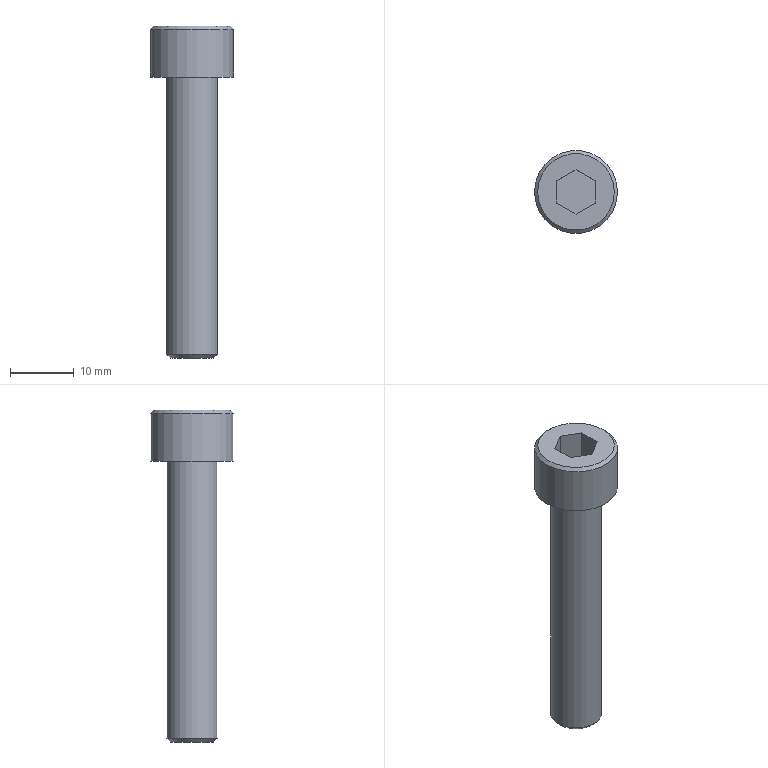Part | STEP file | gslz 2016.10.28-6_id178_x_t | 1 solid | 14 faces | box 13 x 13 x 52 mm | volume 3108 mm3 | plane 10 | cylinder 2 | cone 2 | commonest cylinder face diameters 8 x1 13 x1
STEP:
#1=CARTESIAN_POINT('',(-246.,150.,36.992));
#2=VERTEX_POINT('',#1);
#3=CARTESIAN_POINT('',(-240.,150.,36.992));
#4=DIRECTION('',(0.,0.,-1.));
#5=DIRECTION('',(-1.,0.,0.));
#6=AXIS2_PLACEMENT_3D('',#3,#4,#5);
#7=CIRCLE('',#6,6.);
#8=EDGE_CURVE('',#2,#2,#7,.T.);
#9=ORIENTED_EDGE('',*,*,#8,.F.);
#10=EDGE_LOOP('',(#9));
#11=FACE_BOUND('',#10,.T.);
#12=CARTESIAN_POINT('',(-237.,151.732,36.992));
#13=VERTEX_POINT('',#12);
#14=CARTESIAN_POINT('',(-237.,148.268,36.992));
#15=VERTEX_POINT('',#14);
#16=CARTESIAN_POINT('',(-237.,151.732,36.992));
#17=DIRECTION('',(0.,-1.,0.));
#18=VECTOR('',#17,1.);
#19=LINE('',#16,#18);
#20=EDGE_CURVE('',#13,#15,#19,.T.);
#21=ORIENTED_EDGE('',*,*,#20,.T.);
#22=CARTESIAN_POINT('',(-240.,146.536,36.992));
#23=VERTEX_POINT('',#22);
#24=CARTESIAN_POINT('',(-237.,148.268,36.992));
#25=DIRECTION('',(-0.866,-0.5,0.));
#26=VECTOR('',#25,1.);
#27=LINE('',#24,#26);
#28=EDGE_CURVE('',#15,#23,#27,.T.);
#29=ORIENTED_EDGE('',*,*,#28,.T.);
#30=CARTESIAN_POINT('',(-243.,148.268,36.992));
#31=VERTEX_POINT('',#30);
#32=CARTESIAN_POINT('',(-240.,146.536,36.992));
#33=DIRECTION('',(-0.866,0.5,0.));
#34=VECTOR('',#33,1.);
#35=LINE('',#32,#34);
#36=EDGE_CURVE('',#23,#31,#35,.T.);
#37=ORIENTED_EDGE('',*,*,#36,.T.);
#38=CARTESIAN_POINT('',(-243.,151.732,36.992));
#39=VERTEX_POINT('',#38);
#40=CARTESIAN_POINT('',(-243.,148.268,36.992));
#41=DIRECTION('',(0.,1.,0.));
#42=VECTOR('',#41,1.);
#43=LINE('',#40,#42);
#44=EDGE_CURVE('',#31,#39,#43,.T.);
#45=ORIENTED_EDGE('',*,*,#44,.T.);
#46=CARTESIAN_POINT('',(-240.,153.464,36.992));
#47=VERTEX_POINT('',#46);
#48=CARTESIAN_POINT('',(-243.,151.732,36.992));
#49=DIRECTION('',(0.866,0.5,0.));
#50=VECTOR('',#49,1.);
#51=LINE('',#48,#50);
#52=EDGE_CURVE('',#39,#47,#51,.T.);
#53=ORIENTED_EDGE('',*,*,#52,.T.);
#54=CARTESIAN_POINT('',(-240.,153.464,36.992));
#55=DIRECTION('',(0.866,-0.5,0.));
#56=VECTOR('',#55,1.);
#57=LINE('',#54,#56);
#58=EDGE_CURVE('',#47,#13,#57,.T.);
#59=ORIENTED_EDGE('',*,*,#58,.T.);
#60=EDGE_LOOP('',(#21,#29,#37,#45,#53,#59));
#61=FACE_BOUND('',#60,.T.);
#62=CARTESIAN_POINT('',(-240.,150.,36.992));
#63=DIRECTION('',(0.,0.,1.));
#64=DIRECTION('',(1.,0.,0.));
#65=AXIS2_PLACEMENT_3D('',#62,#63,#64);
#66=PLANE('',#65);
#67=ADVANCED_FACE('',(#11,#61),#66,.T.);
#68=CARTESIAN_POINT('',(-236.6,150.,-15.008));
#69=VERTEX_POINT('',#68);
#70=CARTESIAN_POINT('',(-240.,150.,-15.008));
#71=DIRECTION('',(0.,0.,1.));
#72=DIRECTION('',(1.,0.,0.));
#73=AXIS2_PLACEMENT_3D('',#70,#71,#72);
#74=CIRCLE('',#73,3.4);
#75=EDGE_CURVE('',#69,#69,#74,.T.);
#76=ORIENTED_EDGE('',*,*,#75,.F.);
#77=EDGE_LOOP('',(#76));
#78=FACE_OUTER_BOUND('',#77,.T.);
#79=CARTESIAN_POINT('',(-240.,150.,-15.008));
#80=DIRECTION('',(0.,0.,-1.));
#81=DIRECTION('',(-1.,0.,0.));
#82=AXIS2_PLACEMENT_3D('',#79,#80,#81);
#83=PLANE('',#82);
#84=ADVANCED_FACE('',(#78),#83,.T.);
#85=CARTESIAN_POINT('',(-236.,150.,-14.408));
#86=VERTEX_POINT('',#85);
#87=CARTESIAN_POINT('',(-240.,150.,-14.408));
#88=DIRECTION('',(0.,0.,-1.));
#89=DIRECTION('',(1.,0.,0.));
#90=AXIS2_PLACEMENT_3D('',#87,#88,#89);
#91=CIRCLE('',#90,4.);
#92=EDGE_CURVE('',#86,#86,#91,.T.);
#93=ORIENTED_EDGE('',*,*,#92,.F.);
#94=EDGE_LOOP('',(#93));
#95=FACE_BOUND('',#94,.T.);
#96=CARTESIAN_POINT('',(-236.,150.,28.992));
#97=VERTEX_POINT('',#96);
#98=CARTESIAN_POINT('',(-240.,150.,28.992));
#99=DIRECTION('',(0.,0.,1.));
#100=DIRECTION('',(1.,0.,0.));
#101=AXIS2_PLACEMENT_3D('',#98,#99,#100);
#102=CIRCLE('',#101,4.);
#103=EDGE_CURVE('',#97,#97,#102,.T.);
#104=ORIENTED_EDGE('',*,*,#103,.F.);
#105=EDGE_LOOP('',(#104));
#106=FACE_BOUND('',#105,.T.);
#107=CARTESIAN_POINT('',(-240.,150.,-0.007538));
#108=DIRECTION('',(0.,0.,-1.));
#109=DIRECTION('',(-1.,0.,0.));
#110=AXIS2_PLACEMENT_3D('',#107,#108,#109);
#111=CYLINDRICAL_SURFACE('',#110,4.);
#112=ADVANCED_FACE('',(#95,#106),#111,.T.);
#113=ORIENTED_EDGE('',*,*,#103,.T.);
#114=EDGE_LOOP('',(#113));
#115=FACE_BOUND('',#114,.T.);
#116=CARTESIAN_POINT('',(-233.5,150.,28.992));
#117=VERTEX_POINT('',#116);
#118=CARTESIAN_POINT('',(-240.,150.,28.992));
#119=DIRECTION('',(0.,0.,1.));
#120=DIRECTION('',(1.,0.,0.));
#121=AXIS2_PLACEMENT_3D('',#118,#119,#120);
#122=CIRCLE('',#121,6.5);
#123=EDGE_CURVE('',#117,#117,#122,.T.);
#124=ORIENTED_EDGE('',*,*,#123,.F.);
#125=EDGE_LOOP('',(#124));
#126=FACE_BOUND('',#125,.T.);
#127=CARTESIAN_POINT('',(-240.,150.,28.992));
#128=DIRECTION('',(0.,0.,-1.));
#129=DIRECTION('',(-1.,0.,0.));
#130=AXIS2_PLACEMENT_3D('',#127,#128,#129);
#131=PLANE('',#130);
#132=ADVANCED_FACE('',(#115,#126),#131,.T.);
#133=CARTESIAN_POINT('',(-246.5,150.,36.492));
#134=VERTEX_POINT('',#133);
#135=CARTESIAN_POINT('',(-240.,150.,36.492));
#136=DIRECTION('',(0.,0.,1.));
#137=DIRECTION('',(-1.,0.,0.));
#138=AXIS2_PLACEMENT_3D('',#135,#136,#137);
#139=CIRCLE('',#138,6.5);
#140=EDGE_CURVE('',#134,#134,#139,.T.);
#141=ORIENTED_EDGE('',*,*,#140,.F.);
#142=EDGE_LOOP('',(#141));
#143=FACE_BOUND('',#142,.T.);
#144=ORIENTED_EDGE('',*,*,#123,.T.);
#145=EDGE_LOOP('',(#144));
#146=FACE_BOUND('',#145,.T.);
#147=CARTESIAN_POINT('',(-240.,150.,39.992));
#148=DIRECTION('',(0.,0.,-1.));
#149=DIRECTION('',(-1.,0.,0.));
#150=AXIS2_PLACEMENT_3D('',#147,#148,#149);
#151=CYLINDRICAL_SURFACE('',#150,6.5);
#152=ADVANCED_FACE('',(#143,#146),#151,.T.);
#153=ORIENTED_EDGE('',*,*,#92,.T.);
#154=EDGE_LOOP('',(#153));
#155=FACE_BOUND('',#154,.T.);
#156=ORIENTED_EDGE('',*,*,#75,.T.);
#157=EDGE_LOOP('',(#156));
#158=FACE_BOUND('',#157,.T.);
#159=CARTESIAN_POINT('',(-240.,150.,-15.008));
#160=DIRECTION('',(0.,0.,1.));
#161=DIRECTION('',(-1.,0.,0.));
#162=AXIS2_PLACEMENT_3D('',#159,#160,#161);
#163=CONICAL_SURFACE('',#162,3.4,45.);
#164=ADVANCED_FACE('',(#155,#158),#163,.T.);
#165=ORIENTED_EDGE('',*,*,#20,.F.);
#166=CARTESIAN_POINT('',(-237.,151.732,31.992));
#167=VERTEX_POINT('',#166);
#168=CARTESIAN_POINT('',(-237.,151.732,31.992));
#169=DIRECTION('',(0.,0.,-1.));
#170=VECTOR('',#169,1.);
#171=LINE('',#168,#170);
#172=EDGE_CURVE('',#13,#167,#171,.T.);
#173=ORIENTED_EDGE('',*,*,#172,.T.);
#174=CARTESIAN_POINT('',(-237.,148.268,31.992));
#175=VERTEX_POINT('',#174);
#176=CARTESIAN_POINT('',(-237.,151.732,31.992));
#177=DIRECTION('',(0.,1.,0.));
#178=VECTOR('',#177,1.);
#179=LINE('',#176,#178);
#180=EDGE_CURVE('',#175,#167,#179,.T.);
#181=ORIENTED_EDGE('',*,*,#180,.F.);
#182=CARTESIAN_POINT('',(-237.,148.268,31.992));
#183=DIRECTION('',(0.,0.,-1.));
#184=VECTOR('',#183,1.);
#185=LINE('',#182,#184);
#186=EDGE_CURVE('',#15,#175,#185,.T.);
#187=ORIENTED_EDGE('',*,*,#186,.F.);
#188=EDGE_LOOP('',(#165,#173,#181,#187));
#189=FACE_OUTER_BOUND('',#188,.T.);
#190=CARTESIAN_POINT('',(-237.,151.732,31.992));
#191=DIRECTION('',(1.,0.,0.));
#192=DIRECTION('',(0.,0.,-1.));
#193=AXIS2_PLACEMENT_3D('',#190,#191,#192);
#194=PLANE('',#193);
#195=ADVANCED_FACE('',(#189),#194,.F.);
#196=ORIENTED_EDGE('',*,*,#28,.F.);
#197=ORIENTED_EDGE('',*,*,#186,.T.);
#198=CARTESIAN_POINT('',(-240.,146.536,31.992));
#199=VERTEX_POINT('',#198);
#200=CARTESIAN_POINT('',(-237.,148.268,31.992));
#201=DIRECTION('',(0.866,0.5,0.));
#202=VECTOR('',#201,1.);
#203=LINE('',#200,#202);
#204=EDGE_CURVE('',#199,#175,#203,.T.);
#205=ORIENTED_EDGE('',*,*,#204,.F.);
#206=CARTESIAN_POINT('',(-240.,146.536,31.992));
#207=DIRECTION('',(0.,0.,-1.));
#208=VECTOR('',#207,1.);
#209=LINE('',#206,#208);
#210=EDGE_CURVE('',#23,#199,#209,.T.);
#211=ORIENTED_EDGE('',*,*,#210,.F.);
#212=EDGE_LOOP('',(#196,#197,#205,#211));
#213=FACE_OUTER_BOUND('',#212,.T.);
#214=CARTESIAN_POINT('',(-237.,148.268,31.992));
#215=DIRECTION('',(0.5,-0.866,0.));
#216=DIRECTION('',(0.866,0.5,0.));
#217=AXIS2_PLACEMENT_3D('',#214,#215,#216);
#218=PLANE('',#217);
#219=ADVANCED_FACE('',(#213),#218,.F.);
#220=ORIENTED_EDGE('',*,*,#36,.F.);
#221=ORIENTED_EDGE('',*,*,#210,.T.);
#222=CARTESIAN_POINT('',(-243.,148.268,31.992));
#223=VERTEX_POINT('',#222);
#224=CARTESIAN_POINT('',(-240.,146.536,31.992));
#225=DIRECTION('',(0.866,-0.5,0.));
#226=VECTOR('',#225,1.);
#227=LINE('',#224,#226);
#228=EDGE_CURVE('',#223,#199,#227,.T.);
#229=ORIENTED_EDGE('',*,*,#228,.F.);
#230=CARTESIAN_POINT('',(-243.,148.268,31.992));
#231=DIRECTION('',(0.,0.,-1.));
#232=VECTOR('',#231,1.);
#233=LINE('',#230,#232);
#234=EDGE_CURVE('',#31,#223,#233,.T.);
#235=ORIENTED_EDGE('',*,*,#234,.F.);
#236=EDGE_LOOP('',(#220,#221,#229,#235));
#237=FACE_OUTER_BOUND('',#236,.T.);
#238=CARTESIAN_POINT('',(-240.,146.536,31.992));
#239=DIRECTION('',(-0.5,-0.866,0.));
#240=DIRECTION('',(0.866,-0.5,0.));
#241=AXIS2_PLACEMENT_3D('',#238,#239,#240);
#242=PLANE('',#241);
#243=ADVANCED_FACE('',(#237),#242,.F.);
#244=ORIENTED_EDGE('',*,*,#44,.F.);
#245=ORIENTED_EDGE('',*,*,#234,.T.);
#246=CARTESIAN_POINT('',(-243.,151.732,31.992));
#247=VERTEX_POINT('',#246);
#248=CARTESIAN_POINT('',(-243.,148.268,31.992));
#249=DIRECTION('',(0.,-1.,0.));
#250=VECTOR('',#249,1.);
#251=LINE('',#248,#250);
#252=EDGE_CURVE('',#247,#223,#251,.T.);
#253=ORIENTED_EDGE('',*,*,#252,.F.);
#254=CARTESIAN_POINT('',(-243.,151.732,31.992));
#255=DIRECTION('',(0.,0.,-1.));
#256=VECTOR('',#255,1.);
#257=LINE('',#254,#256);
#258=EDGE_CURVE('',#39,#247,#257,.T.);
#259=ORIENTED_EDGE('',*,*,#258,.F.);
#260=EDGE_LOOP('',(#244,#245,#253,#259));
#261=FACE_OUTER_BOUND('',#260,.T.);
#262=CARTESIAN_POINT('',(-243.,148.268,31.992));
#263=DIRECTION('',(-1.,0.,0.));
#264=DIRECTION('',(0.,0.,1.));
#265=AXIS2_PLACEMENT_3D('',#262,#263,#264);
#266=PLANE('',#265);
#267=ADVANCED_FACE('',(#261),#266,.F.);
#268=ORIENTED_EDGE('',*,*,#52,.F.);
#269=ORIENTED_EDGE('',*,*,#258,.T.);
#270=CARTESIAN_POINT('',(-240.,153.464,31.992));
#271=VERTEX_POINT('',#270);
#272=CARTESIAN_POINT('',(-243.,151.732,31.992));
#273=DIRECTION('',(-0.866,-0.5,0.));
#274=VECTOR('',#273,1.);
#275=LINE('',#272,#274);
#276=EDGE_CURVE('',#271,#247,#275,.T.);
#277=ORIENTED_EDGE('',*,*,#276,.F.);
#278=CARTESIAN_POINT('',(-240.,153.464,31.992));
#279=DIRECTION('',(0.,0.,-1.));
#280=VECTOR('',#279,1.);
#281=LINE('',#278,#280);
#282=EDGE_CURVE('',#47,#271,#281,.T.);
#283=ORIENTED_EDGE('',*,*,#282,.F.);
#284=EDGE_LOOP('',(#268,#269,#277,#283));
#285=FACE_OUTER_BOUND('',#284,.T.);
#286=CARTESIAN_POINT('',(-243.,151.732,31.992));
#287=DIRECTION('',(-0.5,0.866,0.));
#288=DIRECTION('',(-0.866,-0.5,0.));
#289=AXIS2_PLACEMENT_3D('',#286,#287,#288);
#290=PLANE('',#289);
#291=ADVANCED_FACE('',(#285),#290,.F.);
#292=ORIENTED_EDGE('',*,*,#58,.F.);
#293=ORIENTED_EDGE('',*,*,#282,.T.);
#294=CARTESIAN_POINT('',(-240.,153.464,31.992));
#295=DIRECTION('',(-0.866,0.5,0.));
#296=VECTOR('',#295,1.);
#297=LINE('',#294,#296);
#298=EDGE_CURVE('',#167,#271,#297,.T.);
#299=ORIENTED_EDGE('',*,*,#298,.F.);
#300=ORIENTED_EDGE('',*,*,#172,.F.);
#301=EDGE_LOOP('',(#292,#293,#299,#300));
#302=FACE_OUTER_BOUND('',#301,.T.);
#303=CARTESIAN_POINT('',(-240.,153.464,31.992));
#304=DIRECTION('',(0.5,0.866,0.));
#305=DIRECTION('',(-0.866,0.5,0.));
#306=AXIS2_PLACEMENT_3D('',#303,#304,#305);
#307=PLANE('',#306);
#308=ADVANCED_FACE('',(#302),#307,.F.);
#309=ORIENTED_EDGE('',*,*,#180,.T.);
#310=ORIENTED_EDGE('',*,*,#298,.T.);
#311=ORIENTED_EDGE('',*,*,#276,.T.);
#312=ORIENTED_EDGE('',*,*,#252,.T.);
#313=ORIENTED_EDGE('',*,*,#228,.T.);
#314=ORIENTED_EDGE('',*,*,#204,.T.);
#315=EDGE_LOOP('',(#309,#310,#311,#312,#313,#314));
#316=FACE_OUTER_BOUND('',#315,.T.);
#317=CARTESIAN_POINT('',(-237.,148.268,31.992));
#318=DIRECTION('',(0.,0.,1.));
#319=DIRECTION('',(1.,0.,0.));
#320=AXIS2_PLACEMENT_3D('',#317,#318,#319);
#321=PLANE('',#320);
#322=ADVANCED_FACE('',(#316),#321,.T.);
#323=ORIENTED_EDGE('',*,*,#8,.T.);
#324=EDGE_LOOP('',(#323));
#325=FACE_BOUND('',#324,.T.);
#326=ORIENTED_EDGE('',*,*,#140,.T.);
#327=EDGE_LOOP('',(#326));
#328=FACE_BOUND('',#327,.T.);
#329=CARTESIAN_POINT('',(-240.,150.,36.492));
#330=DIRECTION('',(0.,0.,-1.));
#331=DIRECTION('',(-1.,0.,0.));
#332=AXIS2_PLACEMENT_3D('',#329,#330,#331);
#333=CONICAL_SURFACE('',#332,6.5,45.);
#334=ADVANCED_FACE('',(#325,#328),#333,.T.);
#335=CLOSED_SHELL('',(#67,#84,#112,#132,#152,#164,#195,#219,#243,#267,#291,#308,#322,#334));
#336=MANIFOLD_SOLID_BREP('',#335);
#337=(LENGTH_UNIT()NAMED_UNIT(*)SI_UNIT(.MILLI.,.METRE.));
#338=UNCERTAINTY_MEASURE_WITH_UNIT(LENGTH_MEASURE(0.00002),#337,'','');
#339=(NAMED_UNIT(*)PLANE_ANGLE_UNIT()SI_UNIT($,.RADIAN.));
#340=PLANE_ANGLE_MEASURE_WITH_UNIT(PLANE_ANGLE_MEASURE(0.01745),#339);
#341=DIMENSIONAL_EXPONENTS(0.,0.,0.,0.,0.,0.,0.);
#342=(CONVERSION_BASED_UNIT('DEGREE',#340)NAMED_UNIT(#341)PLANE_ANGLE_UNIT());
#343=(NAMED_UNIT(*)SI_UNIT($,.STERADIAN.)SOLID_ANGLE_UNIT());
#344=(GEOMETRIC_REPRESENTATION_CONTEXT(3)GLOBAL_UNCERTAINTY_ASSIGNED_CONTEXT((#338))GLOBAL_UNIT_ASSIGNED_CONTEXT((#337,#342,#343))REPRESENTATION_CONTEXT('',''));
#345=ADVANCED_BREP_SHAPE_REPRESENTATION('',(#336),#344);